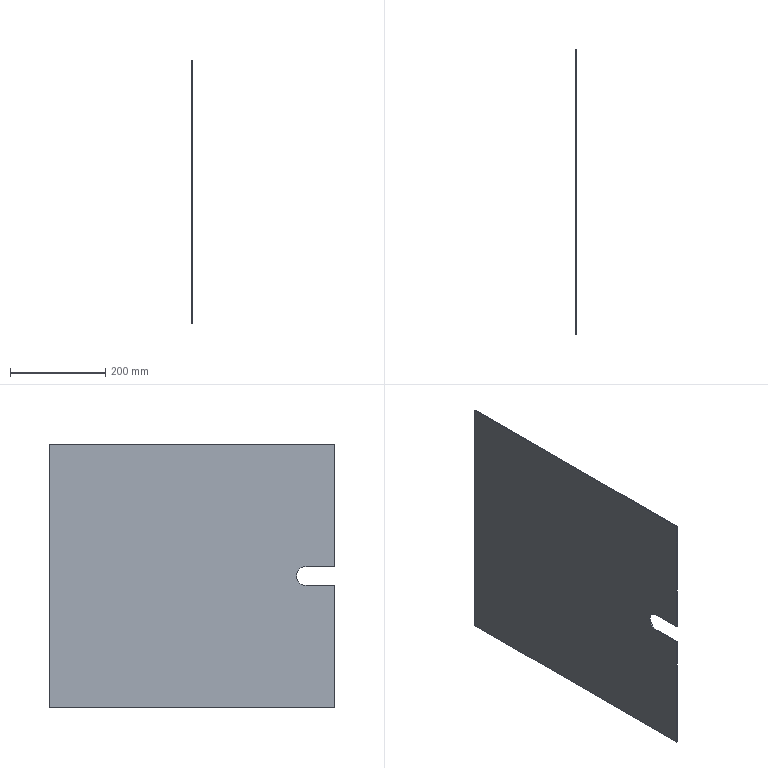Part | SolidWorks | features FlatPattern 1, SMBaseFlange 1, SheetMetal 1 | 1 solid | 10 faces | box 2 x 600 x 554 mm | volume 658743 mm3 | plane 9 | cylinder 1 | commonest cylinder face diameters 40 x1
STEP:
#1=CARTESIAN_POINT('',(0.,-300.,-277.));
#2=VERTEX_POINT('',#1);
#3=CARTESIAN_POINT('',(0.,300.,-277.));
#4=VERTEX_POINT('',#3);
#5=CARTESIAN_POINT('',(0.,-300.,-277.));
#6=DIRECTION('',(0.,1.,0.));
#7=VECTOR('',#6,1000.);
#8=LINE('',#5,#7);
#9=EDGE_CURVE('',#2,#4,#8,.T.);
#10=ORIENTED_EDGE('',*,*,#9,.F.);
#11=CARTESIAN_POINT('',(-2.,-300.,-277.));
#12=VERTEX_POINT('',#11);
#13=CARTESIAN_POINT('',(-2.,-300.,-277.));
#14=DIRECTION('',(1.,0.,0.));
#15=VECTOR('',#14,1000.);
#16=LINE('',#13,#15);
#17=EDGE_CURVE('',#12,#2,#16,.T.);
#18=ORIENTED_EDGE('',*,*,#17,.F.);
#19=CARTESIAN_POINT('',(-2.,300.,-277.));
#20=VERTEX_POINT('',#19);
#21=CARTESIAN_POINT('',(-2.,-300.,-277.));
#22=DIRECTION('',(0.,1.,0.));
#23=VECTOR('',#22,1000.);
#24=LINE('',#21,#23);
#25=EDGE_CURVE('',#12,#20,#24,.T.);
#26=ORIENTED_EDGE('',*,*,#25,.T.);
#27=CARTESIAN_POINT('',(-2.,300.,-277.));
#28=DIRECTION('',(1.,0.,0.));
#29=VECTOR('',#28,1000.);
#30=LINE('',#27,#29);
#31=EDGE_CURVE('',#20,#4,#30,.T.);
#32=ORIENTED_EDGE('',*,*,#31,.T.);
#33=EDGE_LOOP('',(#10,#18,#26,#32));
#34=FACE_OUTER_BOUND('',#33,.T.);
#35=CARTESIAN_POINT('',(-2.,-300.,-277.));
#36=DIRECTION('',(0.,0.,-1.));
#37=DIRECTION('',(-1.,0.,0.));
#38=AXIS2_PLACEMENT_3D('',#35,#36,#37);
#39=PLANE('',#38);
#40=ADVANCED_FACE('',(#34),#39,.T.);
#41=CARTESIAN_POINT('',(0.,-300.,-20.));
#42=VERTEX_POINT('',#41);
#43=CARTESIAN_POINT('',(0.,-300.,-20.));
#44=DIRECTION('',(0.,0.,-1.));
#45=VECTOR('',#44,1000.);
#46=LINE('',#43,#45);
#47=EDGE_CURVE('',#42,#2,#46,.T.);
#48=ORIENTED_EDGE('',*,*,#47,.F.);
#49=CARTESIAN_POINT('',(-2.,-300.,-20.));
#50=VERTEX_POINT('',#49);
#51=CARTESIAN_POINT('',(-2.,-300.,-20.));
#52=DIRECTION('',(1.,0.,0.));
#53=VECTOR('',#52,1000.);
#54=LINE('',#51,#53);
#55=EDGE_CURVE('',#50,#42,#54,.T.);
#56=ORIENTED_EDGE('',*,*,#55,.F.);
#57=CARTESIAN_POINT('',(-2.,-300.,-20.));
#58=DIRECTION('',(0.,0.,-1.));
#59=VECTOR('',#58,1000.);
#60=LINE('',#57,#59);
#61=EDGE_CURVE('',#50,#12,#60,.T.);
#62=ORIENTED_EDGE('',*,*,#61,.T.);
#63=ORIENTED_EDGE('',*,*,#17,.T.);
#64=EDGE_LOOP('',(#48,#56,#62,#63));
#65=FACE_OUTER_BOUND('',#64,.T.);
#66=CARTESIAN_POINT('',(-2.,-300.,-20.));
#67=DIRECTION('',(0.,-1.,0.));
#68=DIRECTION('',(0.,0.,-1.));
#69=AXIS2_PLACEMENT_3D('',#66,#67,#68);
#70=PLANE('',#69);
#71=ADVANCED_FACE('',(#65),#70,.T.);
#72=CARTESIAN_POINT('',(0.,-240.,-20.));
#73=VERTEX_POINT('',#72);
#74=CARTESIAN_POINT('',(0.,-240.,-20.));
#75=DIRECTION('',(0.,-1.,0.));
#76=VECTOR('',#75,1000.);
#77=LINE('',#74,#76);
#78=EDGE_CURVE('',#73,#42,#77,.T.);
#79=ORIENTED_EDGE('',*,*,#78,.F.);
#80=CARTESIAN_POINT('',(-2.,-240.,-20.));
#81=VERTEX_POINT('',#80);
#82=CARTESIAN_POINT('',(-2.,-240.,-20.));
#83=DIRECTION('',(1.,0.,0.));
#84=VECTOR('',#83,1000.);
#85=LINE('',#82,#84);
#86=EDGE_CURVE('',#81,#73,#85,.T.);
#87=ORIENTED_EDGE('',*,*,#86,.F.);
#88=CARTESIAN_POINT('',(-2.,-240.,-20.));
#89=DIRECTION('',(0.,-1.,0.));
#90=VECTOR('',#89,1000.);
#91=LINE('',#88,#90);
#92=EDGE_CURVE('',#81,#50,#91,.T.);
#93=ORIENTED_EDGE('',*,*,#92,.T.);
#94=ORIENTED_EDGE('',*,*,#55,.T.);
#95=EDGE_LOOP('',(#79,#87,#93,#94));
#96=FACE_OUTER_BOUND('',#95,.T.);
#97=CARTESIAN_POINT('',(-2.,-240.,-20.));
#98=DIRECTION('',(0.,0.,1.));
#99=DIRECTION('',(0.,-1.,0.));
#100=AXIS2_PLACEMENT_3D('',#97,#98,#99);
#101=PLANE('',#100);
#102=ADVANCED_FACE('',(#96),#101,.T.);
#103=CARTESIAN_POINT('',(0.,-240.,20.));
#104=VERTEX_POINT('',#103);
#105=CARTESIAN_POINT('',(0.,-240.,0.));
#106=DIRECTION('',(-1.,0.,0.));
#107=DIRECTION('',(0.,0.,-1.));
#108=AXIS2_PLACEMENT_3D('',#105,#106,#107);
#109=CIRCLE('',#108,20.);
#110=EDGE_CURVE('',#104,#73,#109,.T.);
#111=ORIENTED_EDGE('',*,*,#110,.F.);
#112=CARTESIAN_POINT('',(-2.,-240.,20.));
#113=VERTEX_POINT('',#112);
#114=CARTESIAN_POINT('',(-2.,-240.,20.));
#115=DIRECTION('',(1.,0.,0.));
#116=VECTOR('',#115,1000.);
#117=LINE('',#114,#116);
#118=EDGE_CURVE('',#113,#104,#117,.T.);
#119=ORIENTED_EDGE('',*,*,#118,.F.);
#120=CARTESIAN_POINT('',(-2.,-240.,0.));
#121=DIRECTION('',(-1.,0.,0.));
#122=DIRECTION('',(0.,0.,-1.));
#123=AXIS2_PLACEMENT_3D('',#120,#121,#122);
#124=CIRCLE('',#123,20.);
#125=EDGE_CURVE('',#113,#81,#124,.T.);
#126=ORIENTED_EDGE('',*,*,#125,.T.);
#127=ORIENTED_EDGE('',*,*,#86,.T.);
#128=EDGE_LOOP('',(#111,#119,#126,#127));
#129=FACE_OUTER_BOUND('',#128,.T.);
#130=CARTESIAN_POINT('',(-2.,-240.,0.));
#131=DIRECTION('',(1.,0.,0.));
#132=DIRECTION('',(0.,0.,-1.));
#133=AXIS2_PLACEMENT_3D('',#130,#131,#132);
#134=CYLINDRICAL_SURFACE('',#133,20.);
#135=ADVANCED_FACE('',(#129),#134,.F.);
#136=CARTESIAN_POINT('',(0.,-300.,20.));
#137=VERTEX_POINT('',#136);
#138=CARTESIAN_POINT('',(0.,-240.,20.));
#139=DIRECTION('',(0.,1.,0.));
#140=VECTOR('',#139,1000.);
#141=LINE('',#138,#140);
#142=EDGE_CURVE('',#137,#104,#141,.T.);
#143=ORIENTED_EDGE('',*,*,#142,.F.);
#144=CARTESIAN_POINT('',(-2.,-300.,20.));
#145=VERTEX_POINT('',#144);
#146=CARTESIAN_POINT('',(-2.,-300.,20.));
#147=DIRECTION('',(1.,0.,0.));
#148=VECTOR('',#147,1000.);
#149=LINE('',#146,#148);
#150=EDGE_CURVE('',#145,#137,#149,.T.);
#151=ORIENTED_EDGE('',*,*,#150,.F.);
#152=CARTESIAN_POINT('',(-2.,-240.,20.));
#153=DIRECTION('',(0.,1.,0.));
#154=VECTOR('',#153,1000.);
#155=LINE('',#152,#154);
#156=EDGE_CURVE('',#145,#113,#155,.T.);
#157=ORIENTED_EDGE('',*,*,#156,.T.);
#158=ORIENTED_EDGE('',*,*,#118,.T.);
#159=EDGE_LOOP('',(#143,#151,#157,#158));
#160=FACE_OUTER_BOUND('',#159,.T.);
#161=CARTESIAN_POINT('',(-2.,-240.,20.));
#162=DIRECTION('',(0.,0.,-1.));
#163=DIRECTION('',(0.,1.,0.));
#164=AXIS2_PLACEMENT_3D('',#161,#162,#163);
#165=PLANE('',#164);
#166=ADVANCED_FACE('',(#160),#165,.T.);
#167=CARTESIAN_POINT('',(0.,-300.,277.));
#168=VERTEX_POINT('',#167);
#169=CARTESIAN_POINT('',(0.,-300.,277.));
#170=DIRECTION('',(0.,0.,-1.));
#171=VECTOR('',#170,1000.);
#172=LINE('',#169,#171);
#173=EDGE_CURVE('',#168,#137,#172,.T.);
#174=ORIENTED_EDGE('',*,*,#173,.F.);
#175=CARTESIAN_POINT('',(-2.,-300.,277.));
#176=VERTEX_POINT('',#175);
#177=CARTESIAN_POINT('',(-2.,-300.,277.));
#178=DIRECTION('',(1.,0.,0.));
#179=VECTOR('',#178,1000.);
#180=LINE('',#177,#179);
#181=EDGE_CURVE('',#176,#168,#180,.T.);
#182=ORIENTED_EDGE('',*,*,#181,.F.);
#183=CARTESIAN_POINT('',(-2.,-300.,277.));
#184=DIRECTION('',(0.,0.,-1.));
#185=VECTOR('',#184,1000.);
#186=LINE('',#183,#185);
#187=EDGE_CURVE('',#176,#145,#186,.T.);
#188=ORIENTED_EDGE('',*,*,#187,.T.);
#189=ORIENTED_EDGE('',*,*,#150,.T.);
#190=EDGE_LOOP('',(#174,#182,#188,#189));
#191=FACE_OUTER_BOUND('',#190,.T.);
#192=CARTESIAN_POINT('',(-2.,-300.,277.));
#193=DIRECTION('',(0.,-1.,0.));
#194=DIRECTION('',(0.,0.,-1.));
#195=AXIS2_PLACEMENT_3D('',#192,#193,#194);
#196=PLANE('',#195);
#197=ADVANCED_FACE('',(#191),#196,.T.);
#198=CARTESIAN_POINT('',(0.,300.,277.));
#199=VERTEX_POINT('',#198);
#200=CARTESIAN_POINT('',(0.,-300.,277.));
#201=DIRECTION('',(0.,-1.,0.));
#202=VECTOR('',#201,1000.);
#203=LINE('',#200,#202);
#204=EDGE_CURVE('',#199,#168,#203,.T.);
#205=ORIENTED_EDGE('',*,*,#204,.F.);
#206=CARTESIAN_POINT('',(-2.,300.,277.));
#207=VERTEX_POINT('',#206);
#208=CARTESIAN_POINT('',(-2.,300.,277.));
#209=DIRECTION('',(1.,0.,0.));
#210=VECTOR('',#209,1000.);
#211=LINE('',#208,#210);
#212=EDGE_CURVE('',#207,#199,#211,.T.);
#213=ORIENTED_EDGE('',*,*,#212,.F.);
#214=CARTESIAN_POINT('',(-2.,-300.,277.));
#215=DIRECTION('',(0.,-1.,0.));
#216=VECTOR('',#215,1000.);
#217=LINE('',#214,#216);
#218=EDGE_CURVE('',#207,#176,#217,.T.);
#219=ORIENTED_EDGE('',*,*,#218,.T.);
#220=ORIENTED_EDGE('',*,*,#181,.T.);
#221=EDGE_LOOP('',(#205,#213,#219,#220));
#222=FACE_OUTER_BOUND('',#221,.T.);
#223=CARTESIAN_POINT('',(-2.,-300.,277.));
#224=DIRECTION('',(0.,0.,1.));
#225=DIRECTION('',(1.,0.,0.));
#226=AXIS2_PLACEMENT_3D('',#223,#224,#225);
#227=PLANE('',#226);
#228=ADVANCED_FACE('',(#222),#227,.T.);
#229=CARTESIAN_POINT('',(0.,300.,277.));
#230=DIRECTION('',(0.,0.,1.));
#231=VECTOR('',#230,1000.);
#232=LINE('',#229,#231);
#233=EDGE_CURVE('',#4,#199,#232,.T.);
#234=ORIENTED_EDGE('',*,*,#233,.F.);
#235=ORIENTED_EDGE('',*,*,#31,.F.);
#236=CARTESIAN_POINT('',(-2.,300.,277.));
#237=DIRECTION('',(0.,0.,1.));
#238=VECTOR('',#237,1000.);
#239=LINE('',#236,#238);
#240=EDGE_CURVE('',#20,#207,#239,.T.);
#241=ORIENTED_EDGE('',*,*,#240,.T.);
#242=ORIENTED_EDGE('',*,*,#212,.T.);
#243=EDGE_LOOP('',(#234,#235,#241,#242));
#244=FACE_OUTER_BOUND('',#243,.T.);
#245=CARTESIAN_POINT('',(-2.,300.,277.));
#246=DIRECTION('',(0.,1.,0.));
#247=DIRECTION('',(0.,0.,1.));
#248=AXIS2_PLACEMENT_3D('',#245,#246,#247);
#249=PLANE('',#248);
#250=ADVANCED_FACE('',(#244),#249,.T.);
#251=ORIENTED_EDGE('',*,*,#25,.F.);
#252=ORIENTED_EDGE('',*,*,#61,.F.);
#253=ORIENTED_EDGE('',*,*,#92,.F.);
#254=ORIENTED_EDGE('',*,*,#125,.F.);
#255=ORIENTED_EDGE('',*,*,#156,.F.);
#256=ORIENTED_EDGE('',*,*,#187,.F.);
#257=ORIENTED_EDGE('',*,*,#218,.F.);
#258=ORIENTED_EDGE('',*,*,#240,.F.);
#259=EDGE_LOOP('',(#251,#252,#253,#254,#255,#256,#257,#258));
#260=FACE_OUTER_BOUND('',#259,.T.);
#261=CARTESIAN_POINT('',(-2.,-240.,0.));
#262=DIRECTION('',(1.,0.,0.));
#263=DIRECTION('',(0.,0.,-1.));
#264=AXIS2_PLACEMENT_3D('',#261,#262,#263);
#265=PLANE('',#264);
#266=ADVANCED_FACE('',(#260),#265,.F.);
#267=ORIENTED_EDGE('',*,*,#9,.T.);
#268=ORIENTED_EDGE('',*,*,#233,.T.);
#269=ORIENTED_EDGE('',*,*,#204,.T.);
#270=ORIENTED_EDGE('',*,*,#173,.T.);
#271=ORIENTED_EDGE('',*,*,#142,.T.);
#272=ORIENTED_EDGE('',*,*,#110,.T.);
#273=ORIENTED_EDGE('',*,*,#78,.T.);
#274=ORIENTED_EDGE('',*,*,#47,.T.);
#275=EDGE_LOOP('',(#267,#268,#269,#270,#271,#272,#273,#274));
#276=FACE_OUTER_BOUND('',#275,.T.);
#277=CARTESIAN_POINT('',(0.,-240.,0.));
#278=DIRECTION('',(1.,0.,0.));
#279=DIRECTION('',(0.,0.,-1.));
#280=AXIS2_PLACEMENT_3D('',#277,#278,#279);
#281=PLANE('',#280);
#282=ADVANCED_FACE('',(#276),#281,.T.);
#283=CLOSED_SHELL('',(#40,#71,#102,#135,#166,#197,#228,#250,#266,#282));
#284=MANIFOLD_SOLID_BREP('',#283);
#285=CARTESIAN_POINT('',(0.,0.,0.));
#286=DIRECTION('',(0.,0.,1.));
#287=DIRECTION('',(1.,0.,0.));
#288=AXIS2_PLACEMENT_3D('',#285,#286,#287);
#289=(LENGTH_UNIT()NAMED_UNIT(*)SI_UNIT(.MILLI.,.METRE.));
#290=UNCERTAINTY_MEASURE_WITH_UNIT(LENGTH_MEASURE(0.00001),#289,'','');
#291=(NAMED_UNIT(*)PLANE_ANGLE_UNIT()SI_UNIT($,.RADIAN.));
#292=(NAMED_UNIT(*)SI_UNIT($,.STERADIAN.)SOLID_ANGLE_UNIT());
#293=(GEOMETRIC_REPRESENTATION_CONTEXT(3)GLOBAL_UNCERTAINTY_ASSIGNED_CONTEXT((#290))GLOBAL_UNIT_ASSIGNED_CONTEXT((#289,#291,#292))REPRESENTATION_CONTEXT('',''));
#294=ADVANCED_BREP_SHAPE_REPRESENTATION('',(#284,#288),#293);